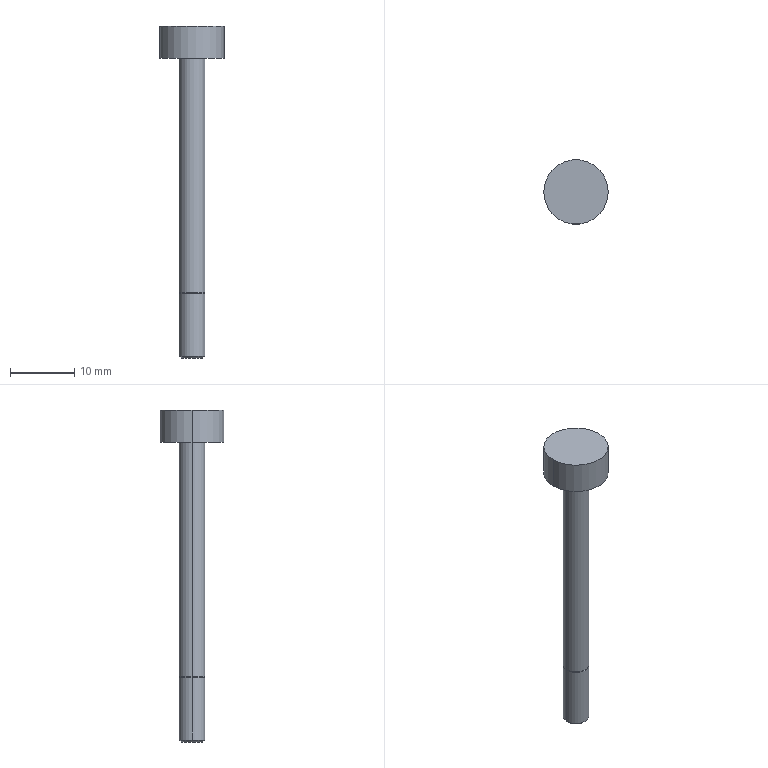Part | NX | 1 solid | 16 faces | box 10 x 10 x 51.5 mm | volume 976.424 mm3 | cylinder 8 | cone 4 | plane 4 | commonest cylinder face diameters 4 x4 3.8 x2 10 x2
STEP:
#1=CARTESIAN_POINT('',(-1.7,0.,-46.5));
#2=VERTEX_POINT('',#1);
#3=CARTESIAN_POINT('',(1.7,0.,-46.5));
#4=VERTEX_POINT('',#3);
#5=CARTESIAN_POINT('',(0.,0.,-46.5));
#6=DIRECTION('',(0.,0.,1.));
#7=DIRECTION('',(1.,0.,0.));
#8=AXIS2_PLACEMENT_3D('',#5,#6,#7);
#9=CIRCLE('',#8,1.7);
#10=EDGE_CURVE('',#2,#4,#9,.T.);
#11=ORIENTED_EDGE('',*,*,#10,.T.);
#12=CARTESIAN_POINT('',(2.,0.,-46.2));
#13=VERTEX_POINT('',#12);
#14=CARTESIAN_POINT('',(2.,0.,-46.2));
#15=DIRECTION('',(0.7071,0.,0.7071));
#16=VECTOR('',#15,1000.);
#17=LINE('',#14,#16);
#18=EDGE_CURVE('',#4,#13,#17,.T.);
#19=ORIENTED_EDGE('',*,*,#18,.T.);
#20=CARTESIAN_POINT('',(-2.,0.,-46.2));
#21=VERTEX_POINT('',#20);
#22=CARTESIAN_POINT('',(0.,0.,-46.2));
#23=DIRECTION('',(0.,0.,1.));
#24=DIRECTION('',(1.,0.,0.));
#25=AXIS2_PLACEMENT_3D('',#22,#23,#24);
#26=CIRCLE('',#25,2.);
#27=EDGE_CURVE('',#21,#13,#26,.T.);
#28=ORIENTED_EDGE('',*,*,#27,.F.);
#29=CARTESIAN_POINT('',(-2.,0.,-46.2));
#30=DIRECTION('',(-0.7071,0.,0.7071));
#31=VECTOR('',#30,1000.);
#32=LINE('',#29,#31);
#33=EDGE_CURVE('',#2,#21,#32,.T.);
#34=ORIENTED_EDGE('',*,*,#33,.F.);
#35=EDGE_LOOP('',(#11,#19,#28,#34));
#36=FACE_BOUND('',#35,.T.);
#37=CARTESIAN_POINT('',(0.,0.,-46.2));
#38=DIRECTION('',(0.,0.,1.));
#39=DIRECTION('',(1.,0.,0.));
#40=AXIS2_PLACEMENT_3D('',#37,#38,#39);
#41=CONICAL_SURFACE('',#40,2.,0.7854);
#42=ADVANCED_FACE('',(#36),#41,.T.);
#43=ORIENTED_EDGE('',*,*,#27,.T.);
#44=CARTESIAN_POINT('',(2.,0.,-36.5));
#45=VERTEX_POINT('',#44);
#46=CARTESIAN_POINT('',(2.,0.,-52.157));
#47=DIRECTION('',(0.,0.,1.));
#48=VECTOR('',#47,1000.);
#49=LINE('',#46,#48);
#50=EDGE_CURVE('',#13,#45,#49,.T.);
#51=ORIENTED_EDGE('',*,*,#50,.T.);
#52=CARTESIAN_POINT('',(-2.,0.,-36.5));
#53=VERTEX_POINT('',#52);
#54=CARTESIAN_POINT('',(0.,0.,-36.5));
#55=DIRECTION('',(0.,0.,1.));
#56=DIRECTION('',(1.,0.,0.));
#57=AXIS2_PLACEMENT_3D('',#54,#55,#56);
#58=CIRCLE('',#57,2.);
#59=EDGE_CURVE('',#53,#45,#58,.T.);
#60=ORIENTED_EDGE('',*,*,#59,.F.);
#61=CARTESIAN_POINT('',(-2.,0.,-52.157));
#62=DIRECTION('',(0.,0.,1.));
#63=VECTOR('',#62,1000.);
#64=LINE('',#61,#63);
#65=EDGE_CURVE('',#21,#53,#64,.T.);
#66=ORIENTED_EDGE('',*,*,#65,.F.);
#67=EDGE_LOOP('',(#43,#51,#60,#66));
#68=FACE_BOUND('',#67,.T.);
#69=CARTESIAN_POINT('',(0.,0.,-52.157));
#70=DIRECTION('',(0.,0.,1.));
#71=DIRECTION('',(1.,0.,0.));
#72=AXIS2_PLACEMENT_3D('',#69,#70,#71);
#73=CYLINDRICAL_SURFACE('',#72,2.);
#74=ADVANCED_FACE('',(#68),#73,.T.);
#75=CARTESIAN_POINT('',(-1.9,0.,-36.49));
#76=VERTEX_POINT('',#75);
#77=CARTESIAN_POINT('',(1.9,0.,-36.49));
#78=VERTEX_POINT('',#77);
#79=CARTESIAN_POINT('',(0.,0.,-36.49));
#80=DIRECTION('',(0.,0.,1.));
#81=DIRECTION('',(1.,0.,0.));
#82=AXIS2_PLACEMENT_3D('',#79,#80,#81);
#83=CIRCLE('',#82,1.9);
#84=EDGE_CURVE('',#76,#78,#83,.T.);
#85=ORIENTED_EDGE('',*,*,#84,.F.);
#86=CARTESIAN_POINT('',(-1.9,0.,-36.5));
#87=VERTEX_POINT('',#86);
#88=CARTESIAN_POINT('',(-1.9,0.,0.));
#89=DIRECTION('',(0.,0.,1.));
#90=VECTOR('',#89,1000.);
#91=LINE('',#88,#90);
#92=EDGE_CURVE('',#76,#87,#91,.F.);
#93=ORIENTED_EDGE('',*,*,#92,.T.);
#94=CARTESIAN_POINT('',(1.9,0.,-36.5));
#95=VERTEX_POINT('',#94);
#96=CARTESIAN_POINT('',(0.,0.,-36.5));
#97=DIRECTION('',(0.,0.,1.));
#98=DIRECTION('',(1.,0.,0.));
#99=AXIS2_PLACEMENT_3D('',#96,#97,#98);
#100=CIRCLE('',#99,1.9);
#101=EDGE_CURVE('',#87,#95,#100,.T.);
#102=ORIENTED_EDGE('',*,*,#101,.T.);
#103=CARTESIAN_POINT('',(1.9,0.,0.));
#104=DIRECTION('',(0.,0.,1.));
#105=VECTOR('',#104,1000.);
#106=LINE('',#103,#105);
#107=EDGE_CURVE('',#78,#95,#106,.F.);
#108=ORIENTED_EDGE('',*,*,#107,.F.);
#109=EDGE_LOOP('',(#85,#93,#102,#108));
#110=FACE_BOUND('',#109,.T.);
#111=CARTESIAN_POINT('',(0.,0.,0.));
#112=DIRECTION('',(0.,0.,1.));
#113=DIRECTION('',(1.,0.,0.));
#114=AXIS2_PLACEMENT_3D('',#111,#112,#113);
#115=CYLINDRICAL_SURFACE('',#114,1.9);
#116=ADVANCED_FACE('',(#110),#115,.T.);
#117=CARTESIAN_POINT('',(-2.,0.,-36.39));
#118=VERTEX_POINT('',#117);
#119=CARTESIAN_POINT('',(2.,0.,-36.39));
#120=VERTEX_POINT('',#119);
#121=CARTESIAN_POINT('',(0.,0.,-36.39));
#122=DIRECTION('',(0.,0.,1.));
#123=DIRECTION('',(1.,0.,0.));
#124=AXIS2_PLACEMENT_3D('',#121,#122,#123);
#125=CIRCLE('',#124,2.);
#126=EDGE_CURVE('',#118,#120,#125,.T.);
#127=ORIENTED_EDGE('',*,*,#126,.F.);
#128=CARTESIAN_POINT('',(-5.,0.,-33.39));
#129=DIRECTION('',(-0.7071,0.,0.7071));
#130=VECTOR('',#129,1000.);
#131=LINE('',#128,#130);
#132=EDGE_CURVE('',#76,#118,#131,.T.);
#133=ORIENTED_EDGE('',*,*,#132,.F.);
#134=ORIENTED_EDGE('',*,*,#84,.T.);
#135=CARTESIAN_POINT('',(5.,0.,-33.39));
#136=DIRECTION('',(0.7071,0.,0.7071));
#137=VECTOR('',#136,1000.);
#138=LINE('',#135,#137);
#139=EDGE_CURVE('',#78,#120,#138,.T.);
#140=ORIENTED_EDGE('',*,*,#139,.T.);
#141=EDGE_LOOP('',(#127,#133,#134,#140));
#142=FACE_BOUND('',#141,.T.);
#143=CARTESIAN_POINT('',(0.,0.,-33.39));
#144=DIRECTION('',(0.,0.,1.));
#145=DIRECTION('',(1.,0.,0.));
#146=AXIS2_PLACEMENT_3D('',#143,#144,#145);
#147=CONICAL_SURFACE('',#146,5.,0.7854);
#148=ADVANCED_FACE('',(#142),#147,.T.);
#149=CARTESIAN_POINT('',(-5.,0.,0.));
#150=VERTEX_POINT('',#149);
#151=CARTESIAN_POINT('',(5.,0.,0.));
#152=VERTEX_POINT('',#151);
#153=CARTESIAN_POINT('',(0.,0.,0.));
#154=DIRECTION('',(0.,0.,1.));
#155=DIRECTION('',(1.,0.,0.));
#156=AXIS2_PLACEMENT_3D('',#153,#154,#155);
#157=CIRCLE('',#156,5.);
#158=EDGE_CURVE('',#150,#152,#157,.T.);
#159=ORIENTED_EDGE('',*,*,#158,.T.);
#160=CARTESIAN_POINT('',(5.,0.,5.));
#161=VERTEX_POINT('',#160);
#162=CARTESIAN_POINT('',(5.,0.,5.));
#163=DIRECTION('',(0.,0.,-1.));
#164=VECTOR('',#163,1000.);
#165=LINE('',#162,#164);
#166=EDGE_CURVE('',#161,#152,#165,.T.);
#167=ORIENTED_EDGE('',*,*,#166,.F.);
#168=CARTESIAN_POINT('',(-5.,0.,5.));
#169=VERTEX_POINT('',#168);
#170=CARTESIAN_POINT('',(0.,0.,5.));
#171=DIRECTION('',(0.,0.,1.));
#172=DIRECTION('',(1.,0.,0.));
#173=AXIS2_PLACEMENT_3D('',#170,#171,#172);
#174=CIRCLE('',#173,5.);
#175=EDGE_CURVE('',#169,#161,#174,.T.);
#176=ORIENTED_EDGE('',*,*,#175,.F.);
#177=CARTESIAN_POINT('',(-5.,0.,5.));
#178=DIRECTION('',(0.,0.,-1.));
#179=VECTOR('',#178,1000.);
#180=LINE('',#177,#179);
#181=EDGE_CURVE('',#169,#150,#180,.T.);
#182=ORIENTED_EDGE('',*,*,#181,.T.);
#183=EDGE_LOOP('',(#159,#167,#176,#182));
#184=FACE_BOUND('',#183,.T.);
#185=CARTESIAN_POINT('',(0.,0.,5.));
#186=DIRECTION('',(0.,0.,-1.));
#187=DIRECTION('',(-1.,0.,0.));
#188=AXIS2_PLACEMENT_3D('',#185,#186,#187);
#189=CYLINDRICAL_SURFACE('',#188,5.);
#190=ADVANCED_FACE('',(#184),#189,.T.);
#191=CARTESIAN_POINT('',(-2.,0.,0.));
#192=VERTEX_POINT('',#191);
#193=CARTESIAN_POINT('',(2.,0.,0.));
#194=VERTEX_POINT('',#193);
#195=CARTESIAN_POINT('',(0.,0.,0.));
#196=DIRECTION('',(0.,0.,1.));
#197=DIRECTION('',(1.,0.,0.));
#198=AXIS2_PLACEMENT_3D('',#195,#196,#197);
#199=CIRCLE('',#198,2.);
#200=EDGE_CURVE('',#192,#194,#199,.T.);
#201=ORIENTED_EDGE('',*,*,#200,.F.);
#202=CARTESIAN_POINT('',(-2.,0.,-52.157));
#203=DIRECTION('',(0.,0.,1.));
#204=VECTOR('',#203,1000.);
#205=LINE('',#202,#204);
#206=EDGE_CURVE('',#118,#192,#205,.T.);
#207=ORIENTED_EDGE('',*,*,#206,.F.);
#208=ORIENTED_EDGE('',*,*,#126,.T.);
#209=CARTESIAN_POINT('',(2.,0.,-52.157));
#210=DIRECTION('',(0.,0.,1.));
#211=VECTOR('',#210,1000.);
#212=LINE('',#209,#211);
#213=EDGE_CURVE('',#120,#194,#212,.T.);
#214=ORIENTED_EDGE('',*,*,#213,.T.);
#215=EDGE_LOOP('',(#201,#207,#208,#214));
#216=FACE_BOUND('',#215,.T.);
#217=CARTESIAN_POINT('',(0.,0.,-52.157));
#218=DIRECTION('',(0.,0.,1.));
#219=DIRECTION('',(1.,0.,0.));
#220=AXIS2_PLACEMENT_3D('',#217,#218,#219);
#221=CYLINDRICAL_SURFACE('',#220,2.);
#222=ADVANCED_FACE('',(#216),#221,.T.);
#223=ORIENTED_EDGE('',*,*,#10,.F.);
#224=CARTESIAN_POINT('',(0.,0.,-46.5));
#225=DIRECTION('',(0.,0.,1.));
#226=DIRECTION('',(1.,0.,0.));
#227=AXIS2_PLACEMENT_3D('',#224,#225,#226);
#228=CIRCLE('',#227,1.7);
#229=EDGE_CURVE('',#4,#2,#228,.T.);
#230=ORIENTED_EDGE('',*,*,#229,.F.);
#231=EDGE_LOOP('',(#223,#230));
#232=FACE_BOUND('',#231,.T.);
#233=CARTESIAN_POINT('',(0.,0.,-46.5));
#234=DIRECTION('',(0.,0.,1.));
#235=DIRECTION('',(1.,0.,0.));
#236=AXIS2_PLACEMENT_3D('',#233,#234,#235);
#237=PLANE('',#236);
#238=ADVANCED_FACE('',(#232),#237,.F.);
#239=CARTESIAN_POINT('',(0.,0.,-36.5));
#240=DIRECTION('',(0.,0.,1.));
#241=DIRECTION('',(1.,0.,0.));
#242=AXIS2_PLACEMENT_3D('',#239,#240,#241);
#243=CIRCLE('',#242,2.);
#244=EDGE_CURVE('',#45,#53,#243,.T.);
#245=ORIENTED_EDGE('',*,*,#244,.T.);
#246=ORIENTED_EDGE('',*,*,#59,.T.);
#247=EDGE_LOOP('',(#245,#246));
#248=FACE_BOUND('',#247,.T.);
#249=CARTESIAN_POINT('',(0.,0.,-36.5));
#250=DIRECTION('',(0.,0.,1.));
#251=DIRECTION('',(1.,0.,0.));
#252=AXIS2_PLACEMENT_3D('',#249,#250,#251);
#253=CIRCLE('',#252,1.9);
#254=EDGE_CURVE('',#95,#87,#253,.T.);
#255=ORIENTED_EDGE('',*,*,#254,.F.);
#256=ORIENTED_EDGE('',*,*,#101,.F.);
#257=EDGE_LOOP('',(#255,#256));
#258=FACE_BOUND('',#257,.T.);
#259=CARTESIAN_POINT('',(0.,2.,-36.5));
#260=DIRECTION('',(0.,0.,1.));
#261=DIRECTION('',(1.,0.,0.));
#262=AXIS2_PLACEMENT_3D('',#259,#260,#261);
#263=PLANE('',#262);
#264=ADVANCED_FACE('',(#248,#258),#263,.T.);
#265=CARTESIAN_POINT('',(0.,0.,5.));
#266=DIRECTION('',(0.,0.,1.));
#267=DIRECTION('',(1.,0.,0.));
#268=AXIS2_PLACEMENT_3D('',#265,#266,#267);
#269=CIRCLE('',#268,5.);
#270=EDGE_CURVE('',#161,#169,#269,.T.);
#271=ORIENTED_EDGE('',*,*,#270,.T.);
#272=ORIENTED_EDGE('',*,*,#175,.T.);
#273=EDGE_LOOP('',(#271,#272));
#274=FACE_BOUND('',#273,.T.);
#275=CARTESIAN_POINT('',(0.,0.,5.));
#276=DIRECTION('',(0.,0.,1.));
#277=DIRECTION('',(1.,0.,0.));
#278=AXIS2_PLACEMENT_3D('',#275,#276,#277);
#279=PLANE('',#278);
#280=ADVANCED_FACE('',(#274),#279,.T.);
#281=ORIENTED_EDGE('',*,*,#158,.F.);
#282=CARTESIAN_POINT('',(0.,0.,0.));
#283=DIRECTION('',(0.,0.,1.));
#284=DIRECTION('',(1.,0.,0.));
#285=AXIS2_PLACEMENT_3D('',#282,#283,#284);
#286=CIRCLE('',#285,5.);
#287=EDGE_CURVE('',#152,#150,#286,.T.);
#288=ORIENTED_EDGE('',*,*,#287,.F.);
#289=EDGE_LOOP('',(#281,#288));
#290=FACE_BOUND('',#289,.T.);
#291=ORIENTED_EDGE('',*,*,#200,.T.);
#292=CARTESIAN_POINT('',(0.,0.,0.));
#293=DIRECTION('',(0.,0.,1.));
#294=DIRECTION('',(1.,0.,0.));
#295=AXIS2_PLACEMENT_3D('',#292,#293,#294);
#296=CIRCLE('',#295,2.);
#297=EDGE_CURVE('',#194,#192,#296,.T.);
#298=ORIENTED_EDGE('',*,*,#297,.T.);
#299=EDGE_LOOP('',(#291,#298));
#300=FACE_BOUND('',#299,.T.);
#301=CARTESIAN_POINT('',(0.,0.,0.));
#302=DIRECTION('',(0.,0.,1.));
#303=DIRECTION('',(1.,0.,0.));
#304=AXIS2_PLACEMENT_3D('',#301,#302,#303);
#305=PLANE('',#304);
#306=ADVANCED_FACE('',(#290,#300),#305,.F.);
#307=ORIENTED_EDGE('',*,*,#244,.F.);
#308=ORIENTED_EDGE('',*,*,#50,.F.);
#309=CARTESIAN_POINT('',(0.,0.,-46.2));
#310=DIRECTION('',(0.,0.,1.));
#311=DIRECTION('',(1.,0.,0.));
#312=AXIS2_PLACEMENT_3D('',#309,#310,#311);
#313=CIRCLE('',#312,2.);
#314=EDGE_CURVE('',#13,#21,#313,.T.);
#315=ORIENTED_EDGE('',*,*,#314,.T.);
#316=ORIENTED_EDGE('',*,*,#65,.T.);
#317=EDGE_LOOP('',(#307,#308,#315,#316));
#318=FACE_BOUND('',#317,.T.);
#319=CARTESIAN_POINT('',(0.,0.,-52.157));
#320=DIRECTION('',(0.,0.,1.));
#321=DIRECTION('',(1.,0.,0.));
#322=AXIS2_PLACEMENT_3D('',#319,#320,#321);
#323=CYLINDRICAL_SURFACE('',#322,2.);
#324=ADVANCED_FACE('',(#318),#323,.T.);
#325=ORIENTED_EDGE('',*,*,#270,.F.);
#326=ORIENTED_EDGE('',*,*,#166,.T.);
#327=ORIENTED_EDGE('',*,*,#287,.T.);
#328=ORIENTED_EDGE('',*,*,#181,.F.);
#329=EDGE_LOOP('',(#325,#326,#327,#328));
#330=FACE_BOUND('',#329,.T.);
#331=CARTESIAN_POINT('',(0.,0.,5.));
#332=DIRECTION('',(0.,0.,-1.));
#333=DIRECTION('',(-1.,0.,0.));
#334=AXIS2_PLACEMENT_3D('',#331,#332,#333);
#335=CYLINDRICAL_SURFACE('',#334,5.);
#336=ADVANCED_FACE('',(#330),#335,.T.);
#337=ORIENTED_EDGE('',*,*,#18,.F.);
#338=ORIENTED_EDGE('',*,*,#229,.T.);
#339=ORIENTED_EDGE('',*,*,#33,.T.);
#340=ORIENTED_EDGE('',*,*,#314,.F.);
#341=EDGE_LOOP('',(#337,#338,#339,#340));
#342=FACE_BOUND('',#341,.T.);
#343=CARTESIAN_POINT('',(0.,0.,-46.2));
#344=DIRECTION('',(0.,0.,1.));
#345=DIRECTION('',(1.,0.,0.));
#346=AXIS2_PLACEMENT_3D('',#343,#344,#345);
#347=CONICAL_SURFACE('',#346,2.,0.7854);
#348=ADVANCED_FACE('',(#342),#347,.T.);
#349=ORIENTED_EDGE('',*,*,#213,.F.);
#350=CARTESIAN_POINT('',(0.,0.,-36.39));
#351=DIRECTION('',(0.,0.,1.));
#352=DIRECTION('',(1.,0.,0.));
#353=AXIS2_PLACEMENT_3D('',#350,#351,#352);
#354=CIRCLE('',#353,2.);
#355=EDGE_CURVE('',#120,#118,#354,.T.);
#356=ORIENTED_EDGE('',*,*,#355,.T.);
#357=ORIENTED_EDGE('',*,*,#206,.T.);
#358=ORIENTED_EDGE('',*,*,#297,.F.);
#359=EDGE_LOOP('',(#349,#356,#357,#358));
#360=FACE_BOUND('',#359,.T.);
#361=CARTESIAN_POINT('',(0.,0.,-52.157));
#362=DIRECTION('',(0.,0.,1.));
#363=DIRECTION('',(1.,0.,0.));
#364=AXIS2_PLACEMENT_3D('',#361,#362,#363);
#365=CYLINDRICAL_SURFACE('',#364,2.);
#366=ADVANCED_FACE('',(#360),#365,.T.);
#367=ORIENTED_EDGE('',*,*,#139,.F.);
#368=CARTESIAN_POINT('',(0.,0.,-36.49));
#369=DIRECTION('',(0.,0.,1.));
#370=DIRECTION('',(1.,0.,0.));
#371=AXIS2_PLACEMENT_3D('',#368,#369,#370);
#372=CIRCLE('',#371,1.9);
#373=EDGE_CURVE('',#78,#76,#372,.T.);
#374=ORIENTED_EDGE('',*,*,#373,.T.);
#375=ORIENTED_EDGE('',*,*,#132,.T.);
#376=ORIENTED_EDGE('',*,*,#355,.F.);
#377=EDGE_LOOP('',(#367,#374,#375,#376));
#378=FACE_BOUND('',#377,.T.);
#379=CARTESIAN_POINT('',(0.,0.,-33.39));
#380=DIRECTION('',(0.,0.,1.));
#381=DIRECTION('',(1.,0.,0.));
#382=AXIS2_PLACEMENT_3D('',#379,#380,#381);
#383=CONICAL_SURFACE('',#382,5.,0.7854);
#384=ADVANCED_FACE('',(#378),#383,.T.);
#385=ORIENTED_EDGE('',*,*,#254,.T.);
#386=ORIENTED_EDGE('',*,*,#92,.F.);
#387=ORIENTED_EDGE('',*,*,#373,.F.);
#388=ORIENTED_EDGE('',*,*,#107,.T.);
#389=EDGE_LOOP('',(#385,#386,#387,#388));
#390=FACE_BOUND('',#389,.T.);
#391=CARTESIAN_POINT('',(0.,0.,0.));
#392=DIRECTION('',(0.,0.,1.));
#393=DIRECTION('',(1.,0.,0.));
#394=AXIS2_PLACEMENT_3D('',#391,#392,#393);
#395=CYLINDRICAL_SURFACE('',#394,1.9);
#396=ADVANCED_FACE('',(#390),#395,.T.);
#397=CLOSED_SHELL('',(#42,#74,#116,#148,#190,#222,#238,#264,#280,#306,#324,#336,#348,#366,#384,#396));
#398=MANIFOLD_SOLID_BREP('',#397);
#399=(LENGTH_UNIT()NAMED_UNIT(*)SI_UNIT(.MILLI.,.METRE.));
#400=UNCERTAINTY_MEASURE_WITH_UNIT(LENGTH_MEASURE(0.00001),#399,'','');
#401=(NAMED_UNIT(*)PLANE_ANGLE_UNIT()SI_UNIT($,.RADIAN.));
#402=(NAMED_UNIT(*)SI_UNIT($,.STERADIAN.)SOLID_ANGLE_UNIT());
#403=(GEOMETRIC_REPRESENTATION_CONTEXT(3)GLOBAL_UNCERTAINTY_ASSIGNED_CONTEXT((#400))GLOBAL_UNIT_ASSIGNED_CONTEXT((#399,#401,#402))REPRESENTATION_CONTEXT('',''));
#404=ADVANCED_BREP_SHAPE_REPRESENTATION('',(#398),#403);